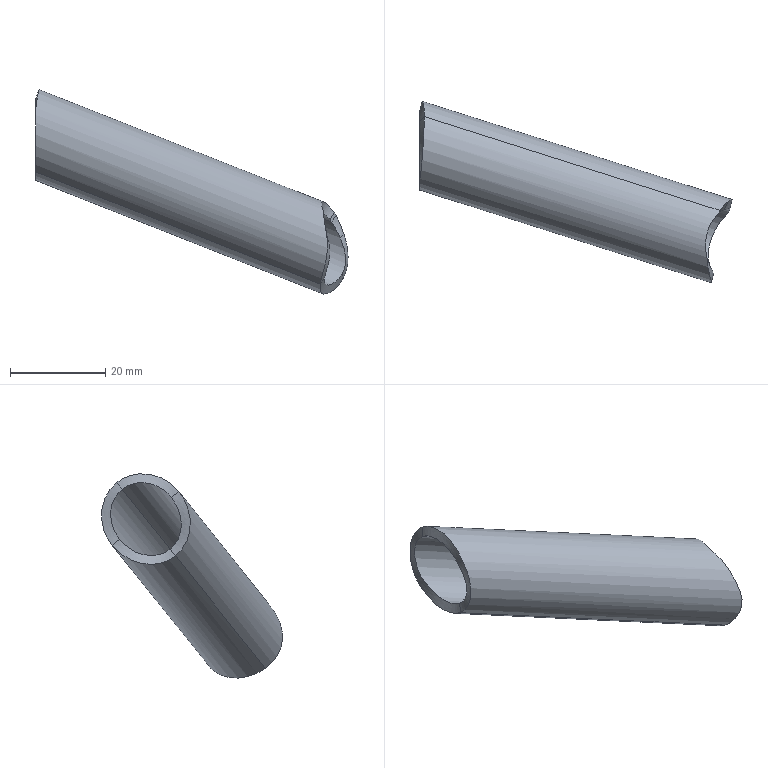Part | SolidWorks | features BaseBody 1 | 1 solid | 14 faces | box 65.619 x 38.058 x 42.973 mm | volume 6942 mm3 | spline 10 | cylinder 4 | commonest cylinder face diameters 14 x2 18 x2